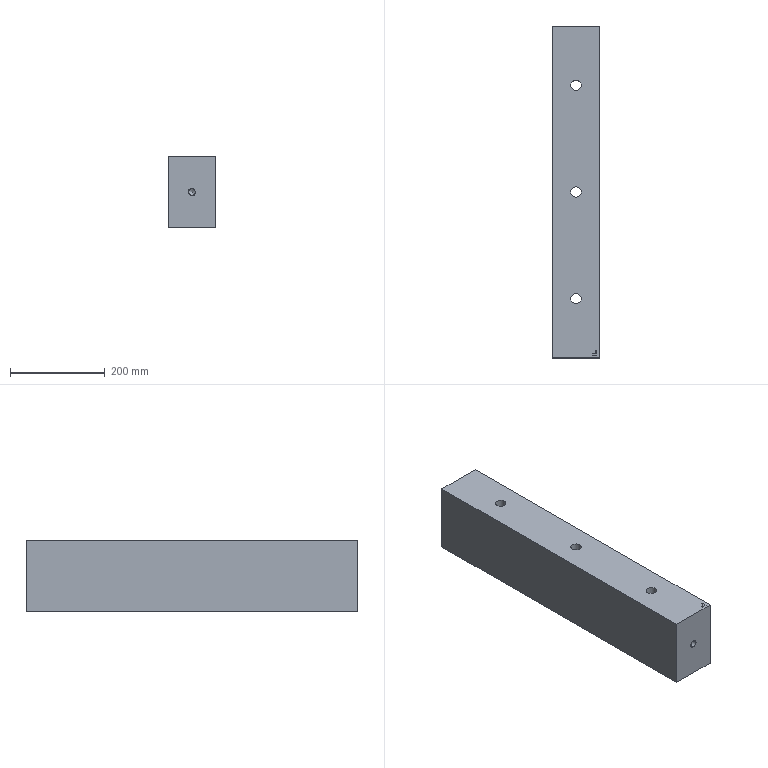Part | NX | features 模具.stp<1>[7] 2 | 1 solid | 48 faces | box 100 x 700 x 150 mm | volume 10309378 mm3 | plane 29 | cylinder 15 | cone 4 | commonest cylinder face diameters 22 x3 12.1 x2 13.7 x2 14 x2 14.1 x2 15.7 x2
STEP:
#1=CARTESIAN_POINT('',(-239.,-225.,-100.5));
#2=VERTEX_POINT('',#1);
#3=CARTESIAN_POINT('',(-250.,-225.,-100.5));
#4=DIRECTION('',(0.,0.,-1.));
#5=DIRECTION('',(1.,0.,0.));
#6=AXIS2_PLACEMENT_3D('',#3,#4,#5);
#7=CIRCLE('',#6,11.);
#8=EDGE_CURVE('',#2,#2,#7,.T.);
#9=ORIENTED_EDGE('',*,*,#8,.F.);
#10=EDGE_LOOP('',(#9));
#11=FACE_BOUND('',#10,.T.);
#12=CARTESIAN_POINT('',(-261.,-225.,-250.5));
#13=VERTEX_POINT('',#12);
#14=CARTESIAN_POINT('',(-250.,-225.,-250.5));
#15=DIRECTION('',(0.,0.,-1.));
#16=DIRECTION('',(-1.,0.,0.));
#17=AXIS2_PLACEMENT_3D('',#14,#15,#16);
#18=CIRCLE('',#17,11.);
#19=EDGE_CURVE('',#13,#13,#18,.T.);
#20=ORIENTED_EDGE('',*,*,#19,.T.);
#21=EDGE_LOOP('',(#20));
#22=FACE_BOUND('',#21,.T.);
#23=CARTESIAN_POINT('',(-250.,-225.,-100.5));
#24=DIRECTION('',(0.,0.,-1.));
#25=DIRECTION('',(1.,0.,0.));
#26=AXIS2_PLACEMENT_3D('',#23,#24,#25);
#27=CYLINDRICAL_SURFACE('',#26,11.);
#28=ADVANCED_FACE('',(#11,#22),#27,.F.);
#29=CARTESIAN_POINT('',(-239.,0.,-100.5));
#30=VERTEX_POINT('',#29);
#31=CARTESIAN_POINT('',(-250.,0.,-100.5));
#32=DIRECTION('',(0.,0.,-1.));
#33=DIRECTION('',(1.,0.,0.));
#34=AXIS2_PLACEMENT_3D('',#31,#32,#33);
#35=CIRCLE('',#34,11.);
#36=EDGE_CURVE('',#30,#30,#35,.T.);
#37=ORIENTED_EDGE('',*,*,#36,.F.);
#38=EDGE_LOOP('',(#37));
#39=FACE_BOUND('',#38,.T.);
#40=CARTESIAN_POINT('',(-261.,0.,-250.5));
#41=VERTEX_POINT('',#40);
#42=CARTESIAN_POINT('',(-250.,0.,-250.5));
#43=DIRECTION('',(0.,0.,-1.));
#44=DIRECTION('',(-1.,0.,0.));
#45=AXIS2_PLACEMENT_3D('',#42,#43,#44);
#46=CIRCLE('',#45,11.);
#47=EDGE_CURVE('',#41,#41,#46,.T.);
#48=ORIENTED_EDGE('',*,*,#47,.T.);
#49=EDGE_LOOP('',(#48));
#50=FACE_BOUND('',#49,.T.);
#51=CARTESIAN_POINT('',(-250.,0.,-100.5));
#52=DIRECTION('',(0.,0.,-1.));
#53=DIRECTION('',(1.,0.,0.));
#54=AXIS2_PLACEMENT_3D('',#51,#52,#53);
#55=CYLINDRICAL_SURFACE('',#54,11.);
#56=ADVANCED_FACE('',(#39,#50),#55,.F.);
#57=CARTESIAN_POINT('',(-239.,225.,-100.5));
#58=VERTEX_POINT('',#57);
#59=CARTESIAN_POINT('',(-250.,225.,-100.5));
#60=DIRECTION('',(0.,0.,-1.));
#61=DIRECTION('',(1.,0.,0.));
#62=AXIS2_PLACEMENT_3D('',#59,#60,#61);
#63=CIRCLE('',#62,11.);
#64=EDGE_CURVE('',#58,#58,#63,.T.);
#65=ORIENTED_EDGE('',*,*,#64,.F.);
#66=EDGE_LOOP('',(#65));
#67=FACE_BOUND('',#66,.T.);
#68=CARTESIAN_POINT('',(-261.,225.,-250.5));
#69=VERTEX_POINT('',#68);
#70=CARTESIAN_POINT('',(-250.,225.,-250.5));
#71=DIRECTION('',(0.,0.,-1.));
#72=DIRECTION('',(-1.,0.,0.));
#73=AXIS2_PLACEMENT_3D('',#70,#71,#72);
#74=CIRCLE('',#73,11.);
#75=EDGE_CURVE('',#69,#69,#74,.T.);
#76=ORIENTED_EDGE('',*,*,#75,.T.);
#77=EDGE_LOOP('',(#76));
#78=FACE_BOUND('',#77,.T.);
#79=CARTESIAN_POINT('',(-250.,225.,-100.5));
#80=DIRECTION('',(0.,0.,-1.));
#81=DIRECTION('',(1.,0.,0.));
#82=AXIS2_PLACEMENT_3D('',#79,#80,#81);
#83=CYLINDRICAL_SURFACE('',#82,11.);
#84=ADVANCED_FACE('',(#67,#78),#83,.F.);
#85=CARTESIAN_POINT('',(-250.,-297.,-215.505));
#86=VERTEX_POINT('',#85);
#87=VERTEX_LOOP('',#86);
#88=FACE_BOUND('',#87,.T.);
#89=CARTESIAN_POINT('',(-243.95,-297.,-218.998));
#90=VERTEX_POINT('',#89);
#91=CARTESIAN_POINT('',(-250.,-297.,-218.998));
#92=DIRECTION('',(0.,0.,1.));
#93=DIRECTION('',(1.,0.,0.));
#94=AXIS2_PLACEMENT_3D('',#91,#92,#93);
#95=CIRCLE('',#94,6.05);
#96=EDGE_CURVE('',#90,#90,#95,.T.);
#97=ORIENTED_EDGE('',*,*,#96,.F.);
#98=EDGE_LOOP('',(#97));
#99=FACE_BOUND('',#98,.T.);
#100=CARTESIAN_POINT('',(-250.,-297.,-216.505));
#101=DIRECTION('',(0.,0.,-1.));
#102=DIRECTION('',(1.,0.,0.));
#103=AXIS2_PLACEMENT_3D('',#100,#101,#102);
#104=CONICAL_SURFACE('',#103,1.732,1.047);
#105=ADVANCED_FACE('',(#88,#99),#104,.F.);
#106=CARTESIAN_POINT('',(-243.95,-297.,-222.5));
#107=VERTEX_POINT('',#106);
#108=CARTESIAN_POINT('',(-243.95,-297.,-223.5));
#109=VERTEX_POINT('',#108);
#110=CARTESIAN_POINT('',(-243.95,-297.,-218.998));
#111=DIRECTION('',(0.,0.,-1.));
#112=VECTOR('',#111,1000.);
#113=LINE('',#110,#112);
#114=EDGE_CURVE('',#107,#109,#113,.T.);
#115=ORIENTED_EDGE('',*,*,#114,.T.);
#116=CARTESIAN_POINT('',(-250.,-303.05,-223.5));
#117=VERTEX_POINT('',#116);
#118=CARTESIAN_POINT('',(-250.,-297.,-223.5));
#119=DIRECTION('',(0.,0.,1.));
#120=DIRECTION('',(0.,-1.,0.));
#121=AXIS2_PLACEMENT_3D('',#118,#119,#120);
#122=CIRCLE('',#121,6.05);
#123=EDGE_CURVE('',#109,#117,#122,.T.);
#124=ORIENTED_EDGE('',*,*,#123,.T.);
#125=CARTESIAN_POINT('',(-250.,-303.05,-222.5));
#126=VERTEX_POINT('',#125);
#127=CARTESIAN_POINT('',(-250.,-303.05,-218.998));
#128=DIRECTION('',(0.,0.,1.));
#129=VECTOR('',#128,1000.);
#130=LINE('',#127,#129);
#131=EDGE_CURVE('',#117,#126,#130,.T.);
#132=ORIENTED_EDGE('',*,*,#131,.T.);
#133=CARTESIAN_POINT('',(-250.,-297.,-222.5));
#134=DIRECTION('',(0.,0.,1.));
#135=DIRECTION('',(0.,-1.,0.));
#136=AXIS2_PLACEMENT_3D('',#133,#134,#135);
#137=CIRCLE('',#136,6.05);
#138=EDGE_CURVE('',#107,#126,#137,.T.);
#139=ORIENTED_EDGE('',*,*,#138,.F.);
#140=EDGE_LOOP('',(#115,#124,#132,#139));
#141=FACE_BOUND('',#140,.T.);
#142=ORIENTED_EDGE('',*,*,#96,.T.);
#143=EDGE_LOOP('',(#142));
#144=FACE_BOUND('',#143,.T.);
#145=CARTESIAN_POINT('',(-256.05,-297.,-250.5));
#146=VERTEX_POINT('',#145);
#147=CARTESIAN_POINT('',(-250.,-297.,-250.5));
#148=DIRECTION('',(0.,0.,-1.));
#149=DIRECTION('',(-1.,0.,0.));
#150=AXIS2_PLACEMENT_3D('',#147,#148,#149);
#151=CIRCLE('',#150,6.05);
#152=EDGE_CURVE('',#146,#146,#151,.T.);
#153=ORIENTED_EDGE('',*,*,#152,.T.);
#154=EDGE_LOOP('',(#153));
#155=FACE_BOUND('',#154,.T.);
#156=CARTESIAN_POINT('',(-250.,-297.,-218.998));
#157=DIRECTION('',(0.,0.,-1.));
#158=DIRECTION('',(1.,0.,0.));
#159=AXIS2_PLACEMENT_3D('',#156,#157,#158);
#160=CYLINDRICAL_SURFACE('',#159,6.05);
#161=ADVANCED_FACE('',(#141,#144,#155),#160,.F.);
#162=CARTESIAN_POINT('',(-250.,-304.,-222.5));
#163=VERTEX_POINT('',#162);
#164=CARTESIAN_POINT('',(-250.,-304.,-250.5));
#165=VERTEX_POINT('',#164);
#166=CARTESIAN_POINT('',(-250.,-304.,-222.5));
#167=DIRECTION('',(0.,0.,-1.));
#168=VECTOR('',#167,1000.);
#169=LINE('',#166,#168);
#170=EDGE_CURVE('',#163,#165,#169,.T.);
#171=ORIENTED_EDGE('',*,*,#170,.F.);
#172=CARTESIAN_POINT('',(-250.,-304.,-222.5));
#173=DIRECTION('',(0.,1.,0.));
#174=VECTOR('',#173,1000.);
#175=LINE('',#172,#174);
#176=EDGE_CURVE('',#163,#126,#175,.T.);
#177=ORIENTED_EDGE('',*,*,#176,.T.);
#178=ORIENTED_EDGE('',*,*,#131,.F.);
#179=CARTESIAN_POINT('',(-250.,-303.85,-223.5));
#180=VERTEX_POINT('',#179);
#181=CARTESIAN_POINT('',(-250.,-297.,-223.5));
#182=DIRECTION('',(0.,-1.,0.));
#183=VECTOR('',#182,1000.);
#184=LINE('',#181,#183);
#185=EDGE_CURVE('',#117,#180,#184,.T.);
#186=ORIENTED_EDGE('',*,*,#185,.T.);
#187=CARTESIAN_POINT('',(-250.,-303.85,-250.5));
#188=VERTEX_POINT('',#187);
#189=CARTESIAN_POINT('',(-250.,-303.85,-223.5));
#190=DIRECTION('',(0.,0.,-1.));
#191=VECTOR('',#190,1000.);
#192=LINE('',#189,#191);
#193=EDGE_CURVE('',#180,#188,#192,.T.);
#194=ORIENTED_EDGE('',*,*,#193,.T.);
#195=CARTESIAN_POINT('',(-250.,0.,-250.5));
#196=DIRECTION('',(0.,1.,0.));
#197=VECTOR('',#196,1000.);
#198=LINE('',#195,#197);
#199=EDGE_CURVE('',#165,#188,#198,.T.);
#200=ORIENTED_EDGE('',*,*,#199,.F.);
#201=EDGE_LOOP('',(#171,#177,#178,#186,#194,#200));
#202=FACE_BOUND('',#201,.T.);
#203=CARTESIAN_POINT('',(-250.,-304.,-222.5));
#204=DIRECTION('',(-1.,0.,0.));
#205=DIRECTION('',(0.,0.,1.));
#206=AXIS2_PLACEMENT_3D('',#203,#204,#205);
#207=PLANE('',#206);
#208=ADVANCED_FACE('',(#202),#207,.T.);
#209=CARTESIAN_POINT('',(-243.15,-297.,-250.5));
#210=VERTEX_POINT('',#209);
#211=CARTESIAN_POINT('',(-243.15,-297.,-223.5));
#212=VERTEX_POINT('',#211);
#213=CARTESIAN_POINT('',(-243.15,-297.,-223.5));
#214=DIRECTION('',(0.,0.,1.));
#215=VECTOR('',#214,1000.);
#216=LINE('',#213,#215);
#217=EDGE_CURVE('',#210,#212,#216,.T.);
#218=ORIENTED_EDGE('',*,*,#217,.T.);
#219=CARTESIAN_POINT('',(-250.,-297.,-223.5));
#220=DIRECTION('',(-1.,0.,0.));
#221=VECTOR('',#220,1000.);
#222=LINE('',#219,#221);
#223=EDGE_CURVE('',#212,#109,#222,.T.);
#224=ORIENTED_EDGE('',*,*,#223,.T.);
#225=ORIENTED_EDGE('',*,*,#114,.F.);
#226=CARTESIAN_POINT('',(-243.,-297.,-222.5));
#227=VERTEX_POINT('',#226);
#228=CARTESIAN_POINT('',(-243.,-297.,-222.5));
#229=DIRECTION('',(1.,0.,0.));
#230=VECTOR('',#229,1000.);
#231=LINE('',#228,#230);
#232=EDGE_CURVE('',#107,#227,#231,.T.);
#233=ORIENTED_EDGE('',*,*,#232,.T.);
#234=CARTESIAN_POINT('',(-243.,-297.,-250.5));
#235=VERTEX_POINT('',#234);
#236=CARTESIAN_POINT('',(-243.,-297.,-222.5));
#237=DIRECTION('',(0.,0.,1.));
#238=VECTOR('',#237,1000.);
#239=LINE('',#236,#238);
#240=EDGE_CURVE('',#235,#227,#239,.T.);
#241=ORIENTED_EDGE('',*,*,#240,.F.);
#242=CARTESIAN_POINT('',(-250.,-297.,-250.5));
#243=DIRECTION('',(1.,0.,0.));
#244=VECTOR('',#243,1000.);
#245=LINE('',#242,#244);
#246=EDGE_CURVE('',#210,#235,#245,.T.);
#247=ORIENTED_EDGE('',*,*,#246,.F.);
#248=EDGE_LOOP('',(#218,#224,#225,#233,#241,#247));
#249=FACE_BOUND('',#248,.T.);
#250=CARTESIAN_POINT('',(-243.,-297.,-222.5));
#251=DIRECTION('',(0.,1.,0.));
#252=DIRECTION('',(0.,0.,-1.));
#253=AXIS2_PLACEMENT_3D('',#250,#251,#252);
#254=PLANE('',#253);
#255=ADVANCED_FACE('',(#249),#254,.T.);
#256=ORIENTED_EDGE('',*,*,#193,.F.);
#257=CARTESIAN_POINT('',(-250.,-297.,-223.5));
#258=DIRECTION('',(0.,0.,-1.));
#259=DIRECTION('',(1.,0.,0.));
#260=AXIS2_PLACEMENT_3D('',#257,#258,#259);
#261=CIRCLE('',#260,6.85);
#262=EDGE_CURVE('',#180,#212,#261,.T.);
#263=ORIENTED_EDGE('',*,*,#262,.T.);
#264=ORIENTED_EDGE('',*,*,#217,.F.);
#265=CARTESIAN_POINT('',(-250.,-297.,-250.5));
#266=DIRECTION('',(0.,0.,-1.));
#267=DIRECTION('',(-1.,0.,0.));
#268=AXIS2_PLACEMENT_3D('',#265,#266,#267);
#269=CIRCLE('',#268,6.85);
#270=EDGE_CURVE('',#188,#210,#269,.T.);
#271=ORIENTED_EDGE('',*,*,#270,.F.);
#272=EDGE_LOOP('',(#256,#263,#264,#271));
#273=FACE_BOUND('',#272,.T.);
#274=CARTESIAN_POINT('',(-250.,-297.,-223.5));
#275=DIRECTION('',(0.,0.,-1.));
#276=DIRECTION('',(1.,0.,0.));
#277=AXIS2_PLACEMENT_3D('',#274,#275,#276);
#278=CYLINDRICAL_SURFACE('',#277,6.85);
#279=ADVANCED_FACE('',(#273),#278,.T.);
#280=ORIENTED_EDGE('',*,*,#223,.F.);
#281=ORIENTED_EDGE('',*,*,#262,.F.);
#282=ORIENTED_EDGE('',*,*,#185,.F.);
#283=ORIENTED_EDGE('',*,*,#123,.F.);
#284=EDGE_LOOP('',(#280,#281,#282,#283));
#285=FACE_BOUND('',#284,.T.);
#286=CARTESIAN_POINT('',(-250.,-297.,-223.5));
#287=DIRECTION('',(0.,0.,1.));
#288=DIRECTION('',(0.,-1.,0.));
#289=AXIS2_PLACEMENT_3D('',#286,#287,#288);
#290=PLANE('',#289);
#291=ADVANCED_FACE('',(#285),#290,.T.);
#292=CARTESIAN_POINT('',(-250.,-297.,-250.5));
#293=DIRECTION('',(0.,0.,-1.));
#294=DIRECTION('',(-1.,0.,0.));
#295=AXIS2_PLACEMENT_3D('',#292,#293,#294);
#296=CIRCLE('',#295,7.);
#297=EDGE_CURVE('',#165,#235,#296,.T.);
#298=ORIENTED_EDGE('',*,*,#297,.T.);
#299=ORIENTED_EDGE('',*,*,#240,.T.);
#300=CARTESIAN_POINT('',(-250.,-297.,-222.5));
#301=DIRECTION('',(0.,0.,-1.));
#302=DIRECTION('',(1.,0.,0.));
#303=AXIS2_PLACEMENT_3D('',#300,#301,#302);
#304=CIRCLE('',#303,7.);
#305=EDGE_CURVE('',#163,#227,#304,.T.);
#306=ORIENTED_EDGE('',*,*,#305,.F.);
#307=ORIENTED_EDGE('',*,*,#170,.T.);
#308=EDGE_LOOP('',(#298,#299,#306,#307));
#309=FACE_BOUND('',#308,.T.);
#310=CARTESIAN_POINT('',(-250.,-297.,-222.5));
#311=DIRECTION('',(0.,0.,-1.));
#312=DIRECTION('',(1.,0.,0.));
#313=AXIS2_PLACEMENT_3D('',#310,#311,#312);
#314=CYLINDRICAL_SURFACE('',#313,7.);
#315=ADVANCED_FACE('',(#309),#314,.F.);
#316=ORIENTED_EDGE('',*,*,#138,.T.);
#317=ORIENTED_EDGE('',*,*,#176,.F.);
#318=ORIENTED_EDGE('',*,*,#305,.T.);
#319=ORIENTED_EDGE('',*,*,#232,.F.);
#320=EDGE_LOOP('',(#316,#317,#318,#319));
#321=FACE_BOUND('',#320,.T.);
#322=CARTESIAN_POINT('',(-250.,-297.,-222.5));
#323=DIRECTION('',(0.,0.,1.));
#324=DIRECTION('',(0.,-1.,0.));
#325=AXIS2_PLACEMENT_3D('',#322,#323,#324);
#326=PLANE('',#325);
#327=ADVANCED_FACE('',(#321),#326,.F.);
#328=CARTESIAN_POINT('',(-250.,297.,-215.505));
#329=VERTEX_POINT('',#328);
#330=VERTEX_LOOP('',#329);
#331=FACE_BOUND('',#330,.T.);
#332=CARTESIAN_POINT('',(-243.95,297.,-218.998));
#333=VERTEX_POINT('',#332);
#334=CARTESIAN_POINT('',(-250.,297.,-218.998));
#335=DIRECTION('',(0.,0.,1.));
#336=DIRECTION('',(1.,0.,0.));
#337=AXIS2_PLACEMENT_3D('',#334,#335,#336);
#338=CIRCLE('',#337,6.05);
#339=EDGE_CURVE('',#333,#333,#338,.T.);
#340=ORIENTED_EDGE('',*,*,#339,.F.);
#341=EDGE_LOOP('',(#340));
#342=FACE_BOUND('',#341,.T.);
#343=CARTESIAN_POINT('',(-250.,297.,-216.505));
#344=DIRECTION('',(0.,0.,-1.));
#345=DIRECTION('',(1.,0.,0.));
#346=AXIS2_PLACEMENT_3D('',#343,#344,#345);
#347=CONICAL_SURFACE('',#346,1.732,1.047);
#348=ADVANCED_FACE('',(#331,#342),#347,.F.);
#349=CARTESIAN_POINT('',(-243.95,297.,-222.5));
#350=VERTEX_POINT('',#349);
#351=CARTESIAN_POINT('',(-243.95,297.,-223.5));
#352=VERTEX_POINT('',#351);
#353=CARTESIAN_POINT('',(-243.95,297.,-218.998));
#354=DIRECTION('',(0.,0.,-1.));
#355=VECTOR('',#354,1000.);
#356=LINE('',#353,#355);
#357=EDGE_CURVE('',#350,#352,#356,.T.);
#358=ORIENTED_EDGE('',*,*,#357,.T.);
#359=CARTESIAN_POINT('',(-250.,290.95,-223.5));
#360=VERTEX_POINT('',#359);
#361=CARTESIAN_POINT('',(-250.,297.,-223.5));
#362=DIRECTION('',(0.,0.,1.));
#363=DIRECTION('',(0.,-1.,0.));
#364=AXIS2_PLACEMENT_3D('',#361,#362,#363);
#365=CIRCLE('',#364,6.05);
#366=EDGE_CURVE('',#352,#360,#365,.T.);
#367=ORIENTED_EDGE('',*,*,#366,.T.);
#368=CARTESIAN_POINT('',(-250.,290.95,-222.5));
#369=VERTEX_POINT('',#368);
#370=CARTESIAN_POINT('',(-250.,290.95,-218.998));
#371=DIRECTION('',(0.,0.,1.));
#372=VECTOR('',#371,1000.);
#373=LINE('',#370,#372);
#374=EDGE_CURVE('',#360,#369,#373,.T.);
#375=ORIENTED_EDGE('',*,*,#374,.T.);
#376=CARTESIAN_POINT('',(-250.,297.,-222.5));
#377=DIRECTION('',(0.,0.,1.));
#378=DIRECTION('',(0.,-1.,0.));
#379=AXIS2_PLACEMENT_3D('',#376,#377,#378);
#380=CIRCLE('',#379,6.05);
#381=EDGE_CURVE('',#350,#369,#380,.T.);
#382=ORIENTED_EDGE('',*,*,#381,.F.);
#383=EDGE_LOOP('',(#358,#367,#375,#382));
#384=FACE_BOUND('',#383,.T.);
#385=ORIENTED_EDGE('',*,*,#339,.T.);
#386=EDGE_LOOP('',(#385));
#387=FACE_BOUND('',#386,.T.);
#388=CARTESIAN_POINT('',(-256.05,297.,-250.5));
#389=VERTEX_POINT('',#388);
#390=CARTESIAN_POINT('',(-250.,297.,-250.5));
#391=DIRECTION('',(0.,0.,-1.));
#392=DIRECTION('',(-1.,0.,0.));
#393=AXIS2_PLACEMENT_3D('',#390,#391,#392);
#394=CIRCLE('',#393,6.05);
#395=EDGE_CURVE('',#389,#389,#394,.T.);
#396=ORIENTED_EDGE('',*,*,#395,.T.);
#397=EDGE_LOOP('',(#396));
#398=FACE_BOUND('',#397,.T.);
#399=CARTESIAN_POINT('',(-250.,297.,-218.998));
#400=DIRECTION('',(0.,0.,-1.));
#401=DIRECTION('',(1.,0.,0.));
#402=AXIS2_PLACEMENT_3D('',#399,#400,#401);
#403=CYLINDRICAL_SURFACE('',#402,6.05);
#404=ADVANCED_FACE('',(#384,#387,#398),#403,.F.);
#405=CARTESIAN_POINT('',(-250.,290.,-222.5));
#406=VERTEX_POINT('',#405);
#407=CARTESIAN_POINT('',(-250.,290.,-250.5));
#408=VERTEX_POINT('',#407);
#409=CARTESIAN_POINT('',(-250.,290.,-222.5));
#410=DIRECTION('',(0.,0.,-1.));
#411=VECTOR('',#410,1000.);
#412=LINE('',#409,#411);
#413=EDGE_CURVE('',#406,#408,#412,.T.);
#414=ORIENTED_EDGE('',*,*,#413,.F.);
#415=CARTESIAN_POINT('',(-250.,290.,-222.5));
#416=DIRECTION('',(0.,1.,0.));
#417=VECTOR('',#416,1000.);
#418=LINE('',#415,#417);
#419=EDGE_CURVE('',#406,#369,#418,.T.);
#420=ORIENTED_EDGE('',*,*,#419,.T.);
#421=ORIENTED_EDGE('',*,*,#374,.F.);
#422=CARTESIAN_POINT('',(-250.,290.15,-223.5));
#423=VERTEX_POINT('',#422);
#424=CARTESIAN_POINT('',(-250.,297.,-223.5));
#425=DIRECTION('',(0.,-1.,0.));
#426=VECTOR('',#425,1000.);
#427=LINE('',#424,#426);
#428=EDGE_CURVE('',#360,#423,#427,.T.);
#429=ORIENTED_EDGE('',*,*,#428,.T.);
#430=CARTESIAN_POINT('',(-250.,290.15,-250.5));
#431=VERTEX_POINT('',#430);
#432=CARTESIAN_POINT('',(-250.,290.15,-223.5));
#433=DIRECTION('',(0.,0.,-1.));
#434=VECTOR('',#433,1000.);
#435=LINE('',#432,#434);
#436=EDGE_CURVE('',#423,#431,#435,.T.);
#437=ORIENTED_EDGE('',*,*,#436,.T.);
#438=CARTESIAN_POINT('',(-250.,0.,-250.5));
#439=DIRECTION('',(0.,1.,0.));
#440=VECTOR('',#439,1000.);
#441=LINE('',#438,#440);
#442=EDGE_CURVE('',#408,#431,#441,.T.);
#443=ORIENTED_EDGE('',*,*,#442,.F.);
#444=EDGE_LOOP('',(#414,#420,#421,#429,#437,#443));
#445=FACE_BOUND('',#444,.T.);
#446=CARTESIAN_POINT('',(-250.,290.,-222.5));
#447=DIRECTION('',(-1.,0.,0.));
#448=DIRECTION('',(0.,0.,1.));
#449=AXIS2_PLACEMENT_3D('',#446,#447,#448);
#450=PLANE('',#449);
#451=ADVANCED_FACE('',(#445),#450,.T.);
#452=CARTESIAN_POINT('',(-243.15,297.,-250.5));
#453=VERTEX_POINT('',#452);
#454=CARTESIAN_POINT('',(-243.15,297.,-223.5));
#455=VERTEX_POINT('',#454);
#456=CARTESIAN_POINT('',(-243.15,297.,-223.5));
#457=DIRECTION('',(0.,0.,1.));
#458=VECTOR('',#457,1000.);
#459=LINE('',#456,#458);
#460=EDGE_CURVE('',#453,#455,#459,.T.);
#461=ORIENTED_EDGE('',*,*,#460,.T.);
#462=CARTESIAN_POINT('',(-250.,297.,-223.5));
#463=DIRECTION('',(-1.,0.,0.));
#464=VECTOR('',#463,1000.);
#465=LINE('',#462,#464);
#466=EDGE_CURVE('',#455,#352,#465,.T.);
#467=ORIENTED_EDGE('',*,*,#466,.T.);
#468=ORIENTED_EDGE('',*,*,#357,.F.);
#469=CARTESIAN_POINT('',(-243.,297.,-222.5));
#470=VERTEX_POINT('',#469);
#471=CARTESIAN_POINT('',(-243.,297.,-222.5));
#472=DIRECTION('',(1.,0.,0.));
#473=VECTOR('',#472,1000.);
#474=LINE('',#471,#473);
#475=EDGE_CURVE('',#350,#470,#474,.T.);
#476=ORIENTED_EDGE('',*,*,#475,.T.);
#477=CARTESIAN_POINT('',(-243.,297.,-250.5));
#478=VERTEX_POINT('',#477);
#479=CARTESIAN_POINT('',(-243.,297.,-222.5));
#480=DIRECTION('',(0.,0.,1.));
#481=VECTOR('',#480,1000.);
#482=LINE('',#479,#481);
#483=EDGE_CURVE('',#478,#470,#482,.T.);
#484=ORIENTED_EDGE('',*,*,#483,.F.);
#485=CARTESIAN_POINT('',(-250.,297.,-250.5));
#486=DIRECTION('',(1.,0.,0.));
#487=VECTOR('',#486,1000.);
#488=LINE('',#485,#487);
#489=EDGE_CURVE('',#453,#478,#488,.T.);
#490=ORIENTED_EDGE('',*,*,#489,.F.);
#491=EDGE_LOOP('',(#461,#467,#468,#476,#484,#490));
#492=FACE_BOUND('',#491,.T.);
#493=CARTESIAN_POINT('',(-243.,297.,-222.5));
#494=DIRECTION('',(0.,1.,0.));
#495=DIRECTION('',(0.,0.,-1.));
#496=AXIS2_PLACEMENT_3D('',#493,#494,#495);
#497=PLANE('',#496);
#498=ADVANCED_FACE('',(#492),#497,.T.);
#499=ORIENTED_EDGE('',*,*,#436,.F.);
#500=CARTESIAN_POINT('',(-250.,297.,-223.5));
#501=DIRECTION('',(0.,0.,-1.));
#502=DIRECTION('',(1.,0.,0.));
#503=AXIS2_PLACEMENT_3D('',#500,#501,#502);
#504=CIRCLE('',#503,6.85);
#505=EDGE_CURVE('',#423,#455,#504,.T.);
#506=ORIENTED_EDGE('',*,*,#505,.T.);
#507=ORIENTED_EDGE('',*,*,#460,.F.);
#508=CARTESIAN_POINT('',(-250.,297.,-250.5));
#509=DIRECTION('',(0.,0.,-1.));
#510=DIRECTION('',(-1.,0.,0.));
#511=AXIS2_PLACEMENT_3D('',#508,#509,#510);
#512=CIRCLE('',#511,6.85);
#513=EDGE_CURVE('',#431,#453,#512,.T.);
#514=ORIENTED_EDGE('',*,*,#513,.F.);
#515=EDGE_LOOP('',(#499,#506,#507,#514));
#516=FACE_BOUND('',#515,.T.);
#517=CARTESIAN_POINT('',(-250.,297.,-223.5));
#518=DIRECTION('',(0.,0.,-1.));
#519=DIRECTION('',(1.,0.,0.));
#520=AXIS2_PLACEMENT_3D('',#517,#518,#519);
#521=CYLINDRICAL_SURFACE('',#520,6.85);
#522=ADVANCED_FACE('',(#516),#521,.T.);
#523=ORIENTED_EDGE('',*,*,#466,.F.);
#524=ORIENTED_EDGE('',*,*,#505,.F.);
#525=ORIENTED_EDGE('',*,*,#428,.F.);
#526=ORIENTED_EDGE('',*,*,#366,.F.);
#527=EDGE_LOOP('',(#523,#524,#525,#526));
#528=FACE_BOUND('',#527,.T.);
#529=CARTESIAN_POINT('',(-250.,297.,-223.5));
#530=DIRECTION('',(0.,0.,1.));
#531=DIRECTION('',(0.,-1.,0.));
#532=AXIS2_PLACEMENT_3D('',#529,#530,#531);
#533=PLANE('',#532);
#534=ADVANCED_FACE('',(#528),#533,.T.);
#535=CARTESIAN_POINT('',(-250.,297.,-250.5));
#536=DIRECTION('',(0.,0.,-1.));
#537=DIRECTION('',(-1.,0.,0.));
#538=AXIS2_PLACEMENT_3D('',#535,#536,#537);
#539=CIRCLE('',#538,7.);
#540=EDGE_CURVE('',#408,#478,#539,.T.);
#541=ORIENTED_EDGE('',*,*,#540,.T.);
#542=ORIENTED_EDGE('',*,*,#483,.T.);
#543=CARTESIAN_POINT('',(-250.,297.,-222.5));
#544=DIRECTION('',(0.,0.,-1.));
#545=DIRECTION('',(1.,0.,0.));
#546=AXIS2_PLACEMENT_3D('',#543,#544,#545);
#547=CIRCLE('',#546,7.);
#548=EDGE_CURVE('',#406,#470,#547,.T.);
#549=ORIENTED_EDGE('',*,*,#548,.F.);
#550=ORIENTED_EDGE('',*,*,#413,.T.);
#551=EDGE_LOOP('',(#541,#542,#549,#550));
#552=FACE_BOUND('',#551,.T.);
#553=CARTESIAN_POINT('',(-250.,297.,-222.5));
#554=DIRECTION('',(0.,0.,-1.));
#555=DIRECTION('',(1.,0.,0.));
#556=AXIS2_PLACEMENT_3D('',#553,#554,#555);
#557=CYLINDRICAL_SURFACE('',#556,7.);
#558=ADVANCED_FACE('',(#552),#557,.F.);
#559=ORIENTED_EDGE('',*,*,#381,.T.);
#560=ORIENTED_EDGE('',*,*,#419,.F.);
#561=ORIENTED_EDGE('',*,*,#548,.T.);
#562=ORIENTED_EDGE('',*,*,#475,.F.);
#563=EDGE_LOOP('',(#559,#560,#561,#562));
#564=FACE_BOUND('',#563,.T.);
#565=CARTESIAN_POINT('',(-250.,297.,-222.5));
#566=DIRECTION('',(0.,0.,1.));
#567=DIRECTION('',(0.,-1.,0.));
#568=AXIS2_PLACEMENT_3D('',#565,#566,#567);
#569=PLANE('',#568);
#570=ADVANCED_FACE('',(#564),#569,.F.);
#571=CARTESIAN_POINT('',(-250.,-311.005,-175.5));
#572=VERTEX_POINT('',#571);
#573=VERTEX_LOOP('',#572);
#574=FACE_BOUND('',#573,.T.);
#575=CARTESIAN_POINT('',(-242.95,-315.075,-175.5));
#576=VERTEX_POINT('',#575);
#577=CARTESIAN_POINT('',(-250.,-315.075,-175.5));
#578=DIRECTION('',(0.,1.,0.));
#579=DIRECTION('',(1.,0.,0.));
#580=AXIS2_PLACEMENT_3D('',#577,#578,#579);
#581=CIRCLE('',#580,7.05);
#582=EDGE_CURVE('',#576,#576,#581,.T.);
#583=ORIENTED_EDGE('',*,*,#582,.F.);
#584=EDGE_LOOP('',(#583));
#585=FACE_BOUND('',#584,.T.);
#586=CARTESIAN_POINT('',(-250.,-312.005,-175.5));
#587=DIRECTION('',(0.,-1.,0.));
#588=DIRECTION('',(1.,0.,0.));
#589=AXIS2_PLACEMENT_3D('',#586,#587,#588);
#590=CONICAL_SURFACE('',#589,1.732,1.047);
#591=ADVANCED_FACE('',(#574,#585),#590,.F.);
#592=CARTESIAN_POINT('',(-242.95,-321.,-175.5));
#593=VERTEX_POINT('',#592);
#594=CARTESIAN_POINT('',(-242.95,-322.,-175.5));
#595=VERTEX_POINT('',#594);
#596=CARTESIAN_POINT('',(-242.95,-315.075,-175.5));
#597=DIRECTION('',(0.,-1.,0.));
#598=VECTOR('',#597,1000.);
#599=LINE('',#596,#598);
#600=EDGE_CURVE('',#593,#595,#599,.T.);
#601=ORIENTED_EDGE('',*,*,#600,.T.);
#602=CARTESIAN_POINT('',(-250.,-322.,-168.45));
#603=VERTEX_POINT('',#602);
#604=CARTESIAN_POINT('',(-250.,-322.,-175.5));
#605=DIRECTION('',(0.,1.,0.));
#606=DIRECTION('',(0.,0.,1.));
#607=AXIS2_PLACEMENT_3D('',#604,#605,#606);
#608=CIRCLE('',#607,7.05);
#609=EDGE_CURVE('',#595,#603,#608,.T.);
#610=ORIENTED_EDGE('',*,*,#609,.T.);
#611=CARTESIAN_POINT('',(-250.,-321.,-168.45));
#612=VERTEX_POINT('',#611);
#613=CARTESIAN_POINT('',(-250.,-315.075,-168.45));
#614=DIRECTION('',(0.,1.,0.));
#615=VECTOR('',#614,1000.);
#616=LINE('',#613,#615);
#617=EDGE_CURVE('',#603,#612,#616,.T.);
#618=ORIENTED_EDGE('',*,*,#617,.T.);
#619=CARTESIAN_POINT('',(-250.,-321.,-175.5));
#620=DIRECTION('',(0.,1.,0.));
#621=DIRECTION('',(0.,0.,1.));
#622=AXIS2_PLACEMENT_3D('',#619,#620,#621);
#623=CIRCLE('',#622,7.05);
#624=EDGE_CURVE('',#593,#612,#623,.T.);
#625=ORIENTED_EDGE('',*,*,#624,.F.);
#626=EDGE_LOOP('',(#601,#610,#618,#625));
#627=FACE_BOUND('',#626,.T.);
#628=ORIENTED_EDGE('',*,*,#582,.T.);
#629=EDGE_LOOP('',(#628));
#630=FACE_BOUND('',#629,.T.);
#631=CARTESIAN_POINT('',(-250.,-350.,-182.55));
#632=VERTEX_POINT('',#631);
#633=CARTESIAN_POINT('',(-250.,-350.,-175.5));
#634=DIRECTION('',(0.,-1.,0.));
#635=DIRECTION('',(0.,0.,-1.));
#636=AXIS2_PLACEMENT_3D('',#633,#634,#635);
#637=CIRCLE('',#636,7.05);
#638=EDGE_CURVE('',#632,#632,#637,.T.);
#639=ORIENTED_EDGE('',*,*,#638,.T.);
#640=EDGE_LOOP('',(#639));
#641=FACE_BOUND('',#640,.T.);
#642=CARTESIAN_POINT('',(-250.,-315.075,-175.5));
#643=DIRECTION('',(0.,-1.,0.));
#644=DIRECTION('',(1.,0.,0.));
#645=AXIS2_PLACEMENT_3D('',#642,#643,#644);
#646=CYLINDRICAL_SURFACE('',#645,7.05);
#647=ADVANCED_FACE('',(#627,#630,#641),#646,.F.);
#648=CARTESIAN_POINT('',(-250.,-321.,-167.5));
#649=VERTEX_POINT('',#648);
#650=CARTESIAN_POINT('',(-250.,-350.,-167.5));
#651=VERTEX_POINT('',#650);
#652=CARTESIAN_POINT('',(-250.,-321.,-167.5));
#653=DIRECTION('',(0.,-1.,0.));
#654=VECTOR('',#653,1000.);
#655=LINE('',#652,#654);
#656=EDGE_CURVE('',#649,#651,#655,.T.);
#657=ORIENTED_EDGE('',*,*,#656,.F.);
#658=CARTESIAN_POINT('',(-250.,-321.,-167.5));
#659=DIRECTION('',(0.,0.,-1.));
#660=VECTOR('',#659,1000.);
#661=LINE('',#658,#660);
#662=EDGE_CURVE('',#649,#612,#661,.T.);
#663=ORIENTED_EDGE('',*,*,#662,.T.);
#664=ORIENTED_EDGE('',*,*,#617,.F.);
#665=CARTESIAN_POINT('',(-250.,-322.,-167.65));
#666=VERTEX_POINT('',#665);
#667=CARTESIAN_POINT('',(-250.,-322.,-175.5));
#668=DIRECTION('',(0.,0.,1.));
#669=VECTOR('',#668,1000.);
#670=LINE('',#667,#669);
#671=EDGE_CURVE('',#603,#666,#670,.T.);
#672=ORIENTED_EDGE('',*,*,#671,.T.);
#673=CARTESIAN_POINT('',(-250.,-350.,-167.65));
#674=VERTEX_POINT('',#673);
#675=CARTESIAN_POINT('',(-250.,-322.,-167.65));
#676=DIRECTION('',(0.,-1.,0.));
#677=VECTOR('',#676,1000.);
#678=LINE('',#675,#677);
#679=EDGE_CURVE('',#666,#674,#678,.T.);
#680=ORIENTED_EDGE('',*,*,#679,.T.);
#681=CARTESIAN_POINT('',(-250.,-350.,-250.5));
#682=DIRECTION('',(0.,0.,-1.));
#683=VECTOR('',#682,1000.);
#684=LINE('',#681,#683);
#685=EDGE_CURVE('',#651,#674,#684,.T.);
#686=ORIENTED_EDGE('',*,*,#685,.F.);
#687=EDGE_LOOP('',(#657,#663,#664,#672,#680,#686));
#688=FACE_BOUND('',#687,.T.);
#689=CARTESIAN_POINT('',(-250.,-321.,-167.5));
#690=DIRECTION('',(-1.,0.,0.));
#691=DIRECTION('',(0.,0.,1.));
#692=AXIS2_PLACEMENT_3D('',#689,#690,#691);
#693=PLANE('',#692);
#694=ADVANCED_FACE('',(#688),#693,.T.);
#695=CARTESIAN_POINT('',(-242.15,-350.,-175.5));
#696=VERTEX_POINT('',#695);
#697=CARTESIAN_POINT('',(-242.15,-322.,-175.5));
#698=VERTEX_POINT('',#697);
#699=CARTESIAN_POINT('',(-242.15,-322.,-175.5));
#700=DIRECTION('',(0.,1.,0.));
#701=VECTOR('',#700,1000.);
#702=LINE('',#699,#701);
#703=EDGE_CURVE('',#696,#698,#702,.T.);
#704=ORIENTED_EDGE('',*,*,#703,.T.);
#705=CARTESIAN_POINT('',(-250.,-322.,-175.5));
#706=DIRECTION('',(-1.,0.,0.));
#707=VECTOR('',#706,1000.);
#708=LINE('',#705,#707);
#709=EDGE_CURVE('',#698,#595,#708,.T.);
#710=ORIENTED_EDGE('',*,*,#709,.T.);
#711=ORIENTED_EDGE('',*,*,#600,.F.);
#712=CARTESIAN_POINT('',(-242.,-321.,-175.5));
#713=VERTEX_POINT('',#712);
#714=CARTESIAN_POINT('',(-242.,-321.,-175.5));
#715=DIRECTION('',(1.,0.,0.));
#716=VECTOR('',#715,1000.);
#717=LINE('',#714,#716);
#718=EDGE_CURVE('',#593,#713,#717,.T.);
#719=ORIENTED_EDGE('',*,*,#718,.T.);
#720=CARTESIAN_POINT('',(-242.,-350.,-175.5));
#721=VERTEX_POINT('',#720);
#722=CARTESIAN_POINT('',(-242.,-321.,-175.5));
#723=DIRECTION('',(0.,1.,0.));
#724=VECTOR('',#723,1000.);
#725=LINE('',#722,#724);
#726=EDGE_CURVE('',#721,#713,#725,.T.);
#727=ORIENTED_EDGE('',*,*,#726,.F.);
#728=CARTESIAN_POINT('',(-250.,-350.,-175.5));
#729=DIRECTION('',(1.,0.,0.));
#730=VECTOR('',#729,1000.);
#731=LINE('',#728,#730);
#732=EDGE_CURVE('',#696,#721,#731,.T.);
#733=ORIENTED_EDGE('',*,*,#732,.F.);
#734=EDGE_LOOP('',(#704,#710,#711,#719,#727,#733));
#735=FACE_BOUND('',#734,.T.);
#736=CARTESIAN_POINT('',(-242.,-321.,-175.5));
#737=DIRECTION('',(0.,0.,-1.));
#738=DIRECTION('',(0.,-1.,0.));
#739=AXIS2_PLACEMENT_3D('',#736,#737,#738);
#740=PLANE('',#739);
#741=ADVANCED_FACE('',(#735),#740,.T.);
#742=ORIENTED_EDGE('',*,*,#679,.F.);
#743=CARTESIAN_POINT('',(-250.,-322.,-175.5));
#744=DIRECTION('',(0.,-1.,0.));
#745=DIRECTION('',(1.,0.,0.));
#746=AXIS2_PLACEMENT_3D('',#743,#744,#745);
#747=CIRCLE('',#746,7.85);
#748=EDGE_CURVE('',#666,#698,#747,.T.);
#749=ORIENTED_EDGE('',*,*,#748,.T.);
#750=ORIENTED_EDGE('',*,*,#703,.F.);
#751=CARTESIAN_POINT('',(-250.,-350.,-175.5));
#752=DIRECTION('',(0.,-1.,0.));
#753=DIRECTION('',(0.,0.,-1.));
#754=AXIS2_PLACEMENT_3D('',#751,#752,#753);
#755=CIRCLE('',#754,7.85);
#756=EDGE_CURVE('',#674,#696,#755,.T.);
#757=ORIENTED_EDGE('',*,*,#756,.F.);
#758=EDGE_LOOP('',(#742,#749,#750,#757));
#759=FACE_BOUND('',#758,.T.);
#760=CARTESIAN_POINT('',(-250.,-322.,-175.5));
#761=DIRECTION('',(0.,-1.,0.));
#762=DIRECTION('',(1.,0.,0.));
#763=AXIS2_PLACEMENT_3D('',#760,#761,#762);
#764=CYLINDRICAL_SURFACE('',#763,7.85);
#765=ADVANCED_FACE('',(#759),#764,.T.);
#766=ORIENTED_EDGE('',*,*,#709,.F.);
#767=ORIENTED_EDGE('',*,*,#748,.F.);
#768=ORIENTED_EDGE('',*,*,#671,.F.);
#769=ORIENTED_EDGE('',*,*,#609,.F.);
#770=EDGE_LOOP('',(#766,#767,#768,#769));
#771=FACE_BOUND('',#770,.T.);
#772=CARTESIAN_POINT('',(-250.,-322.,-175.5));
#773=DIRECTION('',(0.,1.,0.));
#774=DIRECTION('',(0.,0.,-1.));
#775=AXIS2_PLACEMENT_3D('',#772,#773,#774);
#776=PLANE('',#775);
#777=ADVANCED_FACE('',(#771),#776,.T.);
#778=CARTESIAN_POINT('',(-250.,-350.,-175.5));
#779=DIRECTION('',(0.,-1.,0.));
#780=DIRECTION('',(0.,0.,-1.));
#781=AXIS2_PLACEMENT_3D('',#778,#779,#780);
#782=CIRCLE('',#781,8.);
#783=EDGE_CURVE('',#651,#721,#782,.T.);
#784=ORIENTED_EDGE('',*,*,#783,.T.);
#785=ORIENTED_EDGE('',*,*,#726,.T.);
#786=CARTESIAN_POINT('',(-250.,-321.,-175.5));
#787=DIRECTION('',(0.,-1.,0.));
#788=DIRECTION('',(1.,0.,0.));
#789=AXIS2_PLACEMENT_3D('',#786,#787,#788);
#790=CIRCLE('',#789,8.);
#791=EDGE_CURVE('',#649,#713,#790,.T.);
#792=ORIENTED_EDGE('',*,*,#791,.F.);
#793=ORIENTED_EDGE('',*,*,#656,.T.);
#794=EDGE_LOOP('',(#784,#785,#792,#793));
#795=FACE_BOUND('',#794,.T.);
#796=CARTESIAN_POINT('',(-250.,-321.,-175.5));
#797=DIRECTION('',(0.,-1.,0.));
#798=DIRECTION('',(1.,0.,0.));
#799=AXIS2_PLACEMENT_3D('',#796,#797,#798);
#800=CYLINDRICAL_SURFACE('',#799,8.);
#801=ADVANCED_FACE('',(#795),#800,.F.);
#802=ORIENTED_EDGE('',*,*,#624,.T.);
#803=ORIENTED_EDGE('',*,*,#662,.F.);
#804=ORIENTED_EDGE('',*,*,#791,.T.);
#805=ORIENTED_EDGE('',*,*,#718,.F.);
#806=EDGE_LOOP('',(#802,#803,#804,#805));
#807=FACE_BOUND('',#806,.T.);
#808=CARTESIAN_POINT('',(-250.,-321.,-175.5));
#809=DIRECTION('',(0.,1.,0.));
#810=DIRECTION('',(0.,0.,-1.));
#811=AXIS2_PLACEMENT_3D('',#808,#809,#810);
#812=PLANE('',#811);
#813=ADVANCED_FACE('',(#807),#812,.F.);
#814=CARTESIAN_POINT('',(-250.,311.005,-175.5));
#815=VERTEX_POINT('',#814);
#816=VERTEX_LOOP('',#815);
#817=FACE_BOUND('',#816,.T.);
#818=CARTESIAN_POINT('',(-242.95,315.075,-175.5));
#819=VERTEX_POINT('',#818);
#820=CARTESIAN_POINT('',(-250.,315.075,-175.5));
#821=DIRECTION('',(0.,-1.,0.));
#822=DIRECTION('',(1.,0.,0.));
#823=AXIS2_PLACEMENT_3D('',#820,#821,#822);
#824=CIRCLE('',#823,7.05);
#825=EDGE_CURVE('',#819,#819,#824,.T.);
#826=ORIENTED_EDGE('',*,*,#825,.F.);
#827=EDGE_LOOP('',(#826));
#828=FACE_BOUND('',#827,.T.);
#829=CARTESIAN_POINT('',(-250.,312.005,-175.5));
#830=DIRECTION('',(0.,1.,0.));
#831=DIRECTION('',(1.,0.,0.));
#832=AXIS2_PLACEMENT_3D('',#829,#830,#831);
#833=CONICAL_SURFACE('',#832,1.732,1.047);
#834=ADVANCED_FACE('',(#817,#828),#833,.F.);
#835=CARTESIAN_POINT('',(-242.95,321.,-175.5));
#836=VERTEX_POINT('',#835);
#837=CARTESIAN_POINT('',(-242.95,322.,-175.5));
#838=VERTEX_POINT('',#837);
#839=CARTESIAN_POINT('',(-242.95,315.075,-175.5));
#840=DIRECTION('',(0.,1.,0.));
#841=VECTOR('',#840,1000.);
#842=LINE('',#839,#841);
#843=EDGE_CURVE('',#836,#838,#842,.T.);
#844=ORIENTED_EDGE('',*,*,#843,.T.);
#845=CARTESIAN_POINT('',(-250.,322.,-182.55));
#846=VERTEX_POINT('',#845);
#847=CARTESIAN_POINT('',(-250.,322.,-175.5));
#848=DIRECTION('',(0.,-1.,0.));
#849=DIRECTION('',(0.,0.,-1.));
#850=AXIS2_PLACEMENT_3D('',#847,#848,#849);
#851=CIRCLE('',#850,7.05);
#852=EDGE_CURVE('',#838,#846,#851,.T.);
#853=ORIENTED_EDGE('',*,*,#852,.T.);
#854=CARTESIAN_POINT('',(-250.,321.,-182.55));
#855=VERTEX_POINT('',#854);
#856=CARTESIAN_POINT('',(-250.,315.075,-182.55));
#857=DIRECTION('',(0.,-1.,0.));
#858=VECTOR('',#857,1000.);
#859=LINE('',#856,#858);
#860=EDGE_CURVE('',#846,#855,#859,.T.);
#861=ORIENTED_EDGE('',*,*,#860,.T.);
#862=CARTESIAN_POINT('',(-250.,321.,-175.5));
#863=DIRECTION('',(0.,-1.,0.));
#864=DIRECTION('',(0.,0.,-1.));
#865=AXIS2_PLACEMENT_3D('',#862,#863,#864);
#866=CIRCLE('',#865,7.05);
#867=EDGE_CURVE('',#836,#855,#866,.T.);
#868=ORIENTED_EDGE('',*,*,#867,.F.);
#869=EDGE_LOOP('',(#844,#853,#861,#868));
#870=FACE_BOUND('',#869,.T.);
#871=ORIENTED_EDGE('',*,*,#825,.T.);
#872=EDGE_LOOP('',(#871));
#873=FACE_BOUND('',#872,.T.);
#874=CARTESIAN_POINT('',(-250.,350.,-168.45));
#875=VERTEX_POINT('',#874);
#876=CARTESIAN_POINT('',(-250.,350.,-175.5));
#877=DIRECTION('',(0.,1.,0.));
#878=DIRECTION('',(0.,0.,1.));
#879=AXIS2_PLACEMENT_3D('',#876,#877,#878);
#880=CIRCLE('',#879,7.05);
#881=EDGE_CURVE('',#875,#875,#880,.T.);
#882=ORIENTED_EDGE('',*,*,#881,.T.);
#883=EDGE_LOOP('',(#882));
#884=FACE_BOUND('',#883,.T.);
#885=CARTESIAN_POINT('',(-250.,315.075,-175.5));
#886=DIRECTION('',(0.,1.,0.));
#887=DIRECTION('',(1.,0.,0.));
#888=AXIS2_PLACEMENT_3D('',#885,#886,#887);
#889=CYLINDRICAL_SURFACE('',#888,7.05);
#890=ADVANCED_FACE('',(#870,#873,#884),#889,.F.);
#891=CARTESIAN_POINT('',(-250.,321.,-183.5));
#892=VERTEX_POINT('',#891);
#893=CARTESIAN_POINT('',(-250.,350.,-183.5));
#894=VERTEX_POINT('',#893);
#895=CARTESIAN_POINT('',(-250.,321.,-183.5));
#896=DIRECTION('',(0.,1.,0.));
#897=VECTOR('',#896,1000.);
#898=LINE('',#895,#897);
#899=EDGE_CURVE('',#892,#894,#898,.T.);
#900=ORIENTED_EDGE('',*,*,#899,.F.);
#901=CARTESIAN_POINT('',(-250.,321.,-183.5));
#902=DIRECTION('',(0.,0.,1.));
#903=VECTOR('',#902,1000.);
#904=LINE('',#901,#903);
#905=EDGE_CURVE('',#892,#855,#904,.T.);
#906=ORIENTED_EDGE('',*,*,#905,.T.);
#907=ORIENTED_EDGE('',*,*,#860,.F.);
#908=CARTESIAN_POINT('',(-250.,322.,-183.35));
#909=VERTEX_POINT('',#908);
#910=CARTESIAN_POINT('',(-250.,322.,-175.5));
#911=DIRECTION('',(0.,0.,-1.));
#912=VECTOR('',#911,1000.);
#913=LINE('',#910,#912);
#914=EDGE_CURVE('',#846,#909,#913,.T.);
#915=ORIENTED_EDGE('',*,*,#914,.T.);
#916=CARTESIAN_POINT('',(-250.,350.,-183.35));
#917=VERTEX_POINT('',#916);
#918=CARTESIAN_POINT('',(-250.,322.,-183.35));
#919=DIRECTION('',(0.,1.,0.));
#920=VECTOR('',#919,1000.);
#921=LINE('',#918,#920);
#922=EDGE_CURVE('',#909,#917,#921,.T.);
#923=ORIENTED_EDGE('',*,*,#922,.T.);
#924=CARTESIAN_POINT('',(-250.,350.,-250.5));
#925=DIRECTION('',(0.,0.,1.));
#926=VECTOR('',#925,1000.);
#927=LINE('',#924,#926);
#928=EDGE_CURVE('',#894,#917,#927,.T.);
#929=ORIENTED_EDGE('',*,*,#928,.F.);
#930=EDGE_LOOP('',(#900,#906,#907,#915,#923,#929));
#931=FACE_BOUND('',#930,.T.);
#932=CARTESIAN_POINT('',(-250.,321.,-183.5));
#933=DIRECTION('',(-1.,0.,0.));
#934=DIRECTION('',(0.,0.,1.));
#935=AXIS2_PLACEMENT_3D('',#932,#933,#934);
#936=PLANE('',#935);
#937=ADVANCED_FACE('',(#931),#936,.T.);
#938=CARTESIAN_POINT('',(-242.15,350.,-175.5));
#939=VERTEX_POINT('',#938);
#940=CARTESIAN_POINT('',(-242.15,322.,-175.5));
#941=VERTEX_POINT('',#940);
#942=CARTESIAN_POINT('',(-242.15,322.,-175.5));
#943=DIRECTION('',(0.,-1.,0.));
#944=VECTOR('',#943,1000.);
#945=LINE('',#942,#944);
#946=EDGE_CURVE('',#939,#941,#945,.T.);
#947=ORIENTED_EDGE('',*,*,#946,.T.);
#948=CARTESIAN_POINT('',(-250.,322.,-175.5));
#949=DIRECTION('',(-1.,0.,0.));
#950=VECTOR('',#949,1000.);
#951=LINE('',#948,#950);
#952=EDGE_CURVE('',#941,#838,#951,.T.);
#953=ORIENTED_EDGE('',*,*,#952,.T.);
#954=ORIENTED_EDGE('',*,*,#843,.F.);
#955=CARTESIAN_POINT('',(-242.,321.,-175.5));
#956=VERTEX_POINT('',#955);
#957=CARTESIAN_POINT('',(-242.,321.,-175.5));
#958=DIRECTION('',(1.,0.,0.));
#959=VECTOR('',#958,1000.);
#960=LINE('',#957,#959);
#961=EDGE_CURVE('',#836,#956,#960,.T.);
#962=ORIENTED_EDGE('',*,*,#961,.T.);
#963=CARTESIAN_POINT('',(-242.,350.,-175.5));
#964=VERTEX_POINT('',#963);
#965=CARTESIAN_POINT('',(-242.,321.,-175.5));
#966=DIRECTION('',(0.,-1.,0.));
#967=VECTOR('',#966,1000.);
#968=LINE('',#965,#967);
#969=EDGE_CURVE('',#964,#956,#968,.T.);
#970=ORIENTED_EDGE('',*,*,#969,.F.);
#971=CARTESIAN_POINT('',(-250.,350.,-175.5));
#972=DIRECTION('',(1.,0.,0.));
#973=VECTOR('',#972,1000.);
#974=LINE('',#971,#973);
#975=EDGE_CURVE('',#939,#964,#974,.T.);
#976=ORIENTED_EDGE('',*,*,#975,.F.);
#977=EDGE_LOOP('',(#947,#953,#954,#962,#970,#976));
#978=FACE_BOUND('',#977,.T.);
#979=CARTESIAN_POINT('',(-242.,321.,-175.5));
#980=DIRECTION('',(0.,0.,1.));
#981=DIRECTION('',(0.,-1.,0.));
#982=AXIS2_PLACEMENT_3D('',#979,#980,#981);
#983=PLANE('',#982);
#984=ADVANCED_FACE('',(#978),#983,.T.);
#985=ORIENTED_EDGE('',*,*,#922,.F.);
#986=CARTESIAN_POINT('',(-250.,322.,-175.5));
#987=DIRECTION('',(0.,1.,0.));
#988=DIRECTION('',(1.,0.,0.));
#989=AXIS2_PLACEMENT_3D('',#986,#987,#988);
#990=CIRCLE('',#989,7.85);
#991=EDGE_CURVE('',#909,#941,#990,.T.);
#992=ORIENTED_EDGE('',*,*,#991,.T.);
#993=ORIENTED_EDGE('',*,*,#946,.F.);
#994=CARTESIAN_POINT('',(-250.,350.,-175.5));
#995=DIRECTION('',(0.,1.,0.));
#996=DIRECTION('',(0.,0.,1.));
#997=AXIS2_PLACEMENT_3D('',#994,#995,#996);
#998=CIRCLE('',#997,7.85);
#999=EDGE_CURVE('',#917,#939,#998,.T.);
#1000=ORIENTED_EDGE('',*,*,#999,.F.);
#1001=EDGE_LOOP('',(#985,#992,#993,#1000));
#1002=FACE_BOUND('',#1001,.T.);
#1003=CARTESIAN_POINT('',(-250.,322.,-175.5));
#1004=DIRECTION('',(0.,1.,0.));
#1005=DIRECTION('',(1.,0.,0.));
#1006=AXIS2_PLACEMENT_3D('',#1003,#1004,#1005);
#1007=CYLINDRICAL_SURFACE('',#1006,7.85);
#1008=ADVANCED_FACE('',(#1002),#1007,.T.);
#1009=ORIENTED_EDGE('',*,*,#952,.F.);
#1010=ORIENTED_EDGE('',*,*,#991,.F.);
#1011=ORIENTED_EDGE('',*,*,#914,.F.);
#1012=ORIENTED_EDGE('',*,*,#852,.F.);
#1013=EDGE_LOOP('',(#1009,#1010,#1011,#1012));
#1014=FACE_BOUND('',#1013,.T.);
#1015=CARTESIAN_POINT('',(-250.,322.,-175.5));
#1016=DIRECTION('',(0.,-1.,0.));
#1017=DIRECTION('',(0.,0.,-1.));
#1018=AXIS2_PLACEMENT_3D('',#1015,#1016,#1017);
#1019=PLANE('',#1018);
#1020=ADVANCED_FACE('',(#1014),#1019,.T.);
#1021=CARTESIAN_POINT('',(-250.,350.,-175.5));
#1022=DIRECTION('',(0.,1.,0.));
#1023=DIRECTION('',(0.,0.,1.));
#1024=AXIS2_PLACEMENT_3D('',#1021,#1022,#1023);
#1025=CIRCLE('',#1024,8.);
#1026=EDGE_CURVE('',#894,#964,#1025,.T.);
#1027=ORIENTED_EDGE('',*,*,#1026,.T.);
#1028=ORIENTED_EDGE('',*,*,#969,.T.);
#1029=CARTESIAN_POINT('',(-250.,321.,-175.5));
#1030=DIRECTION('',(0.,1.,0.));
#1031=DIRECTION('',(1.,0.,0.));
#1032=AXIS2_PLACEMENT_3D('',#1029,#1030,#1031);
#1033=CIRCLE('',#1032,8.);
#1034=EDGE_CURVE('',#892,#956,#1033,.T.);
#1035=ORIENTED_EDGE('',*,*,#1034,.F.);
#1036=ORIENTED_EDGE('',*,*,#899,.T.);
#1037=EDGE_LOOP('',(#1027,#1028,#1035,#1036));
#1038=FACE_BOUND('',#1037,.T.);
#1039=CARTESIAN_POINT('',(-250.,321.,-175.5));
#1040=DIRECTION('',(0.,1.,0.));
#1041=DIRECTION('',(1.,0.,0.));
#1042=AXIS2_PLACEMENT_3D('',#1039,#1040,#1041);
#1043=CYLINDRICAL_SURFACE('',#1042,8.);
#1044=ADVANCED_FACE('',(#1038),#1043,.F.);
#1045=ORIENTED_EDGE('',*,*,#867,.T.);
#1046=ORIENTED_EDGE('',*,*,#905,.F.);
#1047=ORIENTED_EDGE('',*,*,#1034,.T.);
#1048=ORIENTED_EDGE('',*,*,#961,.F.);
#1049=EDGE_LOOP('',(#1045,#1046,#1047,#1048));
#1050=FACE_BOUND('',#1049,.T.);
#1051=CARTESIAN_POINT('',(-250.,321.,-175.5));
#1052=DIRECTION('',(0.,-1.,0.));
#1053=DIRECTION('',(0.,0.,-1.));
#1054=AXIS2_PLACEMENT_3D('',#1051,#1052,#1053);
#1055=PLANE('',#1054);
#1056=ADVANCED_FACE('',(#1050),#1055,.F.);
#1057=CARTESIAN_POINT('',(-216.,-344.,-100.8));
#1058=VERTEX_POINT('',#1057);
#1059=CARTESIAN_POINT('',(-206.,-344.,-100.8));
#1060=VERTEX_POINT('',#1059);
#1061=CARTESIAN_POINT('',(-216.,-344.,-100.8));
#1062=DIRECTION('',(1.,0.,0.));
#1063=VECTOR('',#1062,1000.);
#1064=LINE('',#1061,#1063);
#1065=EDGE_CURVE('',#1058,#1060,#1064,.T.);
#1066=ORIENTED_EDGE('',*,*,#1065,.T.);
#1067=CARTESIAN_POINT('',(-206.,-334.,-100.8));
#1068=VERTEX_POINT('',#1067);
#1069=CARTESIAN_POINT('',(-206.,-334.,-100.8));
#1070=DIRECTION('',(0.,1.,0.));
#1071=VECTOR('',#1070,1000.);
#1072=LINE('',#1069,#1071);
#1073=EDGE_CURVE('',#1060,#1068,#1072,.T.);
#1074=ORIENTED_EDGE('',*,*,#1073,.T.);
#1075=CARTESIAN_POINT('',(-209.,-334.,-100.8));
#1076=VERTEX_POINT('',#1075);
#1077=CARTESIAN_POINT('',(-209.,-334.,-100.8));
#1078=DIRECTION('',(-1.,0.,0.));
#1079=VECTOR('',#1078,1000.);
#1080=LINE('',#1077,#1079);
#1081=EDGE_CURVE('',#1068,#1076,#1080,.T.);
#1082=ORIENTED_EDGE('',*,*,#1081,.T.);
#1083=CARTESIAN_POINT('',(-209.,-341.,-100.8));
#1084=VERTEX_POINT('',#1083);
#1085=CARTESIAN_POINT('',(-209.,-341.,-100.8));
#1086=DIRECTION('',(0.,-1.,0.));
#1087=VECTOR('',#1086,1000.);
#1088=LINE('',#1085,#1087);
#1089=EDGE_CURVE('',#1076,#1084,#1088,.T.);
#1090=ORIENTED_EDGE('',*,*,#1089,.T.);
#1091=CARTESIAN_POINT('',(-216.,-341.,-100.8));
#1092=VERTEX_POINT('',#1091);
#1093=CARTESIAN_POINT('',(-216.,-341.,-100.8));
#1094=DIRECTION('',(-1.,0.,0.));
#1095=VECTOR('',#1094,1000.);
#1096=LINE('',#1093,#1095);
#1097=EDGE_CURVE('',#1084,#1092,#1096,.T.);
#1098=ORIENTED_EDGE('',*,*,#1097,.T.);
#1099=CARTESIAN_POINT('',(-216.,-344.,-100.8));
#1100=DIRECTION('',(0.,-1.,0.));
#1101=VECTOR('',#1100,1000.);
#1102=LINE('',#1099,#1101);
#1103=EDGE_CURVE('',#1092,#1058,#1102,.T.);
#1104=ORIENTED_EDGE('',*,*,#1103,.T.);
#1105=EDGE_LOOP('',(#1066,#1074,#1082,#1090,#1098,#1104));
#1106=FACE_BOUND('',#1105,.T.);
#1107=CARTESIAN_POINT('',(-206.,-344.,-100.8));
#1108=DIRECTION('',(0.,0.,1.));
#1109=DIRECTION('',(1.,0.,0.));
#1110=AXIS2_PLACEMENT_3D('',#1107,#1108,#1109);
#1111=PLANE('',#1110);
#1112=ADVANCED_FACE('',(#1106),#1111,.T.);
#1113=CARTESIAN_POINT('',(-216.,-341.,-100.5));
#1114=VERTEX_POINT('',#1113);
#1115=CARTESIAN_POINT('',(-216.,-344.,-100.5));
#1116=VERTEX_POINT('',#1115);
#1117=CARTESIAN_POINT('',(-216.,-344.,-100.5));
#1118=DIRECTION('',(0.,-1.,0.));
#1119=VECTOR('',#1118,1000.);
#1120=LINE('',#1117,#1119);
#1121=EDGE_CURVE('',#1114,#1116,#1120,.T.);
#1122=ORIENTED_EDGE('',*,*,#1121,.T.);
#1123=CARTESIAN_POINT('',(-216.,-344.,-100.8));
#1124=DIRECTION('',(0.,0.,1.));
#1125=VECTOR('',#1124,1000.);
#1126=LINE('',#1123,#1125);
#1127=EDGE_CURVE('',#1058,#1116,#1126,.T.);
#1128=ORIENTED_EDGE('',*,*,#1127,.F.);
#1129=ORIENTED_EDGE('',*,*,#1103,.F.);
#1130=CARTESIAN_POINT('',(-216.,-341.,-100.8));
#1131=DIRECTION('',(0.,0.,1.));
#1132=VECTOR('',#1131,1000.);
#1133=LINE('',#1130,#1132);
#1134=EDGE_CURVE('',#1092,#1114,#1133,.T.);
#1135=ORIENTED_EDGE('',*,*,#1134,.T.);
#1136=EDGE_LOOP('',(#1122,#1128,#1129,#1135));
#1137=FACE_BOUND('',#1136,.T.);
#1138=CARTESIAN_POINT('',(-216.,-344.,-100.8));
#1139=DIRECTION('',(-1.,0.,0.));
#1140=DIRECTION('',(0.,0.,1.));
#1141=AXIS2_PLACEMENT_3D('',#1138,#1139,#1140);
#1142=PLANE('',#1141);
#1143=ADVANCED_FACE('',(#1137),#1142,.F.);
#1144=CARTESIAN_POINT('',(-209.,-341.,-100.5));
#1145=VERTEX_POINT('',#1144);
#1146=CARTESIAN_POINT('',(-216.,-341.,-100.5));
#1147=DIRECTION('',(-1.,0.,0.));
#1148=VECTOR('',#1147,1000.);
#1149=LINE('',#1146,#1148);
#1150=EDGE_CURVE('',#1145,#1114,#1149,.T.);
#1151=ORIENTED_EDGE('',*,*,#1150,.T.);
#1152=ORIENTED_EDGE('',*,*,#1134,.F.);
#1153=ORIENTED_EDGE('',*,*,#1097,.F.);
#1154=CARTESIAN_POINT('',(-209.,-341.,-100.8));
#1155=DIRECTION('',(0.,0.,1.));
#1156=VECTOR('',#1155,1000.);
#1157=LINE('',#1154,#1156);
#1158=EDGE_CURVE('',#1084,#1145,#1157,.T.);
#1159=ORIENTED_EDGE('',*,*,#1158,.T.);
#1160=EDGE_LOOP('',(#1151,#1152,#1153,#1159));
#1161=FACE_BOUND('',#1160,.T.);
#1162=CARTESIAN_POINT('',(-216.,-341.,-100.8));
#1163=DIRECTION('',(0.,1.,0.));
#1164=DIRECTION('',(1.,0.,0.));
#1165=AXIS2_PLACEMENT_3D('',#1162,#1163,#1164);
#1166=PLANE('',#1165);
#1167=ADVANCED_FACE('',(#1161),#1166,.F.);
#1168=CARTESIAN_POINT('',(-209.,-334.,-100.5));
#1169=VERTEX_POINT('',#1168);
#1170=CARTESIAN_POINT('',(-209.,-341.,-100.5));
#1171=DIRECTION('',(0.,-1.,0.));
#1172=VECTOR('',#1171,1000.);
#1173=LINE('',#1170,#1172);
#1174=EDGE_CURVE('',#1169,#1145,#1173,.T.);
#1175=ORIENTED_EDGE('',*,*,#1174,.T.);
#1176=ORIENTED_EDGE('',*,*,#1158,.F.);
#1177=ORIENTED_EDGE('',*,*,#1089,.F.);
#1178=CARTESIAN_POINT('',(-209.,-334.,-100.8));
#1179=DIRECTION('',(0.,0.,1.));
#1180=VECTOR('',#1179,1000.);
#1181=LINE('',#1178,#1180);
#1182=EDGE_CURVE('',#1076,#1169,#1181,.T.);
#1183=ORIENTED_EDGE('',*,*,#1182,.T.);
#1184=EDGE_LOOP('',(#1175,#1176,#1177,#1183));
#1185=FACE_BOUND('',#1184,.T.);
#1186=CARTESIAN_POINT('',(-209.,-341.,-100.8));
#1187=DIRECTION('',(-1.,0.,0.));
#1188=DIRECTION('',(0.,0.,1.));
#1189=AXIS2_PLACEMENT_3D('',#1186,#1187,#1188);
#1190=PLANE('',#1189);
#1191=ADVANCED_FACE('',(#1185),#1190,.F.);
#1192=CARTESIAN_POINT('',(-206.,-334.,-100.5));
#1193=VERTEX_POINT('',#1192);
#1194=CARTESIAN_POINT('',(-209.,-334.,-100.5));
#1195=DIRECTION('',(-1.,0.,0.));
#1196=VECTOR('',#1195,1000.);
#1197=LINE('',#1194,#1196);
#1198=EDGE_CURVE('',#1193,#1169,#1197,.T.);
#1199=ORIENTED_EDGE('',*,*,#1198,.T.);
#1200=ORIENTED_EDGE('',*,*,#1182,.F.);
#1201=ORIENTED_EDGE('',*,*,#1081,.F.);
#1202=CARTESIAN_POINT('',(-206.,-334.,-100.8));
#1203=DIRECTION('',(0.,0.,1.));
#1204=VECTOR('',#1203,1000.);
#1205=LINE('',#1202,#1204);
#1206=EDGE_CURVE('',#1068,#1193,#1205,.T.);
#1207=ORIENTED_EDGE('',*,*,#1206,.T.);
#1208=EDGE_LOOP('',(#1199,#1200,#1201,#1207));
#1209=FACE_BOUND('',#1208,.T.);
#1210=CARTESIAN_POINT('',(-209.,-334.,-100.8));
#1211=DIRECTION('',(0.,1.,0.));
#1212=DIRECTION('',(1.,0.,0.));
#1213=AXIS2_PLACEMENT_3D('',#1210,#1211,#1212);
#1214=PLANE('',#1213);
#1215=ADVANCED_FACE('',(#1209),#1214,.F.);
#1216=CARTESIAN_POINT('',(-206.,-344.,-100.5));
#1217=VERTEX_POINT('',#1216);
#1218=CARTESIAN_POINT('',(-206.,-334.,-100.5));
#1219=DIRECTION('',(0.,1.,0.));
#1220=VECTOR('',#1219,1000.);
#1221=LINE('',#1218,#1220);
#1222=EDGE_CURVE('',#1217,#1193,#1221,.T.);
#1223=ORIENTED_EDGE('',*,*,#1222,.T.);
#1224=ORIENTED_EDGE('',*,*,#1206,.F.);
#1225=ORIENTED_EDGE('',*,*,#1073,.F.);
#1226=CARTESIAN_POINT('',(-206.,-344.,-100.8));
#1227=DIRECTION('',(0.,0.,1.));
#1228=VECTOR('',#1227,1000.);
#1229=LINE('',#1226,#1228);
#1230=EDGE_CURVE('',#1060,#1217,#1229,.T.);
#1231=ORIENTED_EDGE('',*,*,#1230,.T.);
#1232=EDGE_LOOP('',(#1223,#1224,#1225,#1231));
#1233=FACE_BOUND('',#1232,.T.);
#1234=CARTESIAN_POINT('',(-206.,-334.,-100.8));
#1235=DIRECTION('',(1.,0.,0.));
#1236=DIRECTION('',(0.,1.,0.));
#1237=AXIS2_PLACEMENT_3D('',#1234,#1235,#1236);
#1238=PLANE('',#1237);
#1239=ADVANCED_FACE('',(#1233),#1238,.F.);
#1240=CARTESIAN_POINT('',(-216.,-344.,-100.5));
#1241=DIRECTION('',(1.,0.,0.));
#1242=VECTOR('',#1241,1000.);
#1243=LINE('',#1240,#1242);
#1244=EDGE_CURVE('',#1116,#1217,#1243,.T.);
#1245=ORIENTED_EDGE('',*,*,#1244,.T.);
#1246=ORIENTED_EDGE('',*,*,#1230,.F.);
#1247=ORIENTED_EDGE('',*,*,#1065,.F.);
#1248=ORIENTED_EDGE('',*,*,#1127,.T.);
#1249=EDGE_LOOP('',(#1245,#1246,#1247,#1248));
#1250=FACE_BOUND('',#1249,.T.);
#1251=CARTESIAN_POINT('',(-216.,-344.,-100.8));
#1252=DIRECTION('',(0.,-1.,0.));
#1253=DIRECTION('',(0.,0.,-1.));
#1254=AXIS2_PLACEMENT_3D('',#1251,#1252,#1253);
#1255=PLANE('',#1254);
#1256=ADVANCED_FACE('',(#1250),#1255,.F.);
#1257=CARTESIAN_POINT('',(-200.,-350.,-250.5));
#1258=VERTEX_POINT('',#1257);
#1259=CARTESIAN_POINT('',(-200.,350.,-250.5));
#1260=VERTEX_POINT('',#1259);
#1261=CARTESIAN_POINT('',(-200.,0.,-250.5));
#1262=DIRECTION('',(0.,1.,0.));
#1263=VECTOR('',#1262,1000.);
#1264=LINE('',#1261,#1263);
#1265=EDGE_CURVE('',#1258,#1260,#1264,.T.);
#1266=ORIENTED_EDGE('',*,*,#1265,.T.);
#1267=CARTESIAN_POINT('',(-200.,350.,-100.5));
#1268=VERTEX_POINT('',#1267);
#1269=CARTESIAN_POINT('',(-200.,350.,-250.5));
#1270=DIRECTION('',(0.,0.,1.));
#1271=VECTOR('',#1270,1000.);
#1272=LINE('',#1269,#1271);
#1273=EDGE_CURVE('',#1260,#1268,#1272,.T.);
#1274=ORIENTED_EDGE('',*,*,#1273,.T.);
#1275=CARTESIAN_POINT('',(-200.,-350.,-100.5));
#1276=VERTEX_POINT('',#1275);
#1277=CARTESIAN_POINT('',(-200.,0.,-100.5));
#1278=DIRECTION('',(0.,-1.,0.));
#1279=VECTOR('',#1278,1000.);
#1280=LINE('',#1277,#1279);
#1281=EDGE_CURVE('',#1268,#1276,#1280,.T.);
#1282=ORIENTED_EDGE('',*,*,#1281,.T.);
#1283=CARTESIAN_POINT('',(-200.,-350.,-250.5));
#1284=DIRECTION('',(0.,0.,1.));
#1285=VECTOR('',#1284,1000.);
#1286=LINE('',#1283,#1285);
#1287=EDGE_CURVE('',#1258,#1276,#1286,.T.);
#1288=ORIENTED_EDGE('',*,*,#1287,.F.);
#1289=EDGE_LOOP('',(#1266,#1274,#1282,#1288));
#1290=FACE_BOUND('',#1289,.T.);
#1291=CARTESIAN_POINT('',(-200.,0.,-250.5));
#1292=DIRECTION('',(1.,0.,0.));
#1293=DIRECTION('',(0.,1.,0.));
#1294=AXIS2_PLACEMENT_3D('',#1291,#1292,#1293);
#1295=PLANE('',#1294);
#1296=ADVANCED_FACE('',(#1290),#1295,.T.);
#1297=CARTESIAN_POINT('',(-300.,-350.,-250.5));
#1298=VERTEX_POINT('',#1297);
#1299=CARTESIAN_POINT('',(-300.,-350.,-100.5));
#1300=VERTEX_POINT('',#1299);
#1301=CARTESIAN_POINT('',(-300.,-350.,-250.5));
#1302=DIRECTION('',(0.,0.,1.));
#1303=VECTOR('',#1302,1000.);
#1304=LINE('',#1301,#1303);
#1305=EDGE_CURVE('',#1298,#1300,#1304,.T.);
#1306=ORIENTED_EDGE('',*,*,#1305,.T.);
#1307=CARTESIAN_POINT('',(-300.,350.,-100.5));
#1308=VERTEX_POINT('',#1307);
#1309=CARTESIAN_POINT('',(-300.,0.,-100.5));
#1310=DIRECTION('',(0.,1.,0.));
#1311=VECTOR('',#1310,1000.);
#1312=LINE('',#1309,#1311);
#1313=EDGE_CURVE('',#1300,#1308,#1312,.T.);
#1314=ORIENTED_EDGE('',*,*,#1313,.T.);
#1315=CARTESIAN_POINT('',(-300.,350.,-250.5));
#1316=VERTEX_POINT('',#1315);
#1317=CARTESIAN_POINT('',(-300.,350.,-250.5));
#1318=DIRECTION('',(0.,0.,1.));
#1319=VECTOR('',#1318,1000.);
#1320=LINE('',#1317,#1319);
#1321=EDGE_CURVE('',#1316,#1308,#1320,.T.);
#1322=ORIENTED_EDGE('',*,*,#1321,.F.);
#1323=CARTESIAN_POINT('',(-300.,0.,-250.5));
#1324=DIRECTION('',(0.,-1.,0.));
#1325=VECTOR('',#1324,1000.);
#1326=LINE('',#1323,#1325);
#1327=EDGE_CURVE('',#1316,#1298,#1326,.T.);
#1328=ORIENTED_EDGE('',*,*,#1327,.T.);
#1329=EDGE_LOOP('',(#1306,#1314,#1322,#1328));
#1330=FACE_BOUND('',#1329,.T.);
#1331=CARTESIAN_POINT('',(-300.,0.,-250.5));
#1332=DIRECTION('',(-1.,0.,0.));
#1333=DIRECTION('',(0.,0.,1.));
#1334=AXIS2_PLACEMENT_3D('',#1331,#1332,#1333);
#1335=PLANE('',#1334);
#1336=ADVANCED_FACE('',(#1330),#1335,.T.);
#1337=CARTESIAN_POINT('',(-250.,-350.,-100.5));
#1338=DIRECTION('',(-1.,0.,0.));
#1339=VECTOR('',#1338,1000.);
#1340=LINE('',#1337,#1339);
#1341=EDGE_CURVE('',#1276,#1300,#1340,.T.);
#1342=ORIENTED_EDGE('',*,*,#1341,.F.);
#1343=ORIENTED_EDGE('',*,*,#1281,.F.);
#1344=CARTESIAN_POINT('',(-250.,350.,-100.5));
#1345=DIRECTION('',(1.,0.,0.));
#1346=VECTOR('',#1345,1000.);
#1347=LINE('',#1344,#1346);
#1348=EDGE_CURVE('',#1308,#1268,#1347,.T.);
#1349=ORIENTED_EDGE('',*,*,#1348,.F.);
#1350=ORIENTED_EDGE('',*,*,#1313,.F.);
#1351=EDGE_LOOP('',(#1342,#1343,#1349,#1350));
#1352=FACE_BOUND('',#1351,.T.);
#1353=ORIENTED_EDGE('',*,*,#1244,.F.);
#1354=ORIENTED_EDGE('',*,*,#1121,.F.);
#1355=ORIENTED_EDGE('',*,*,#1150,.F.);
#1356=ORIENTED_EDGE('',*,*,#1174,.F.);
#1357=ORIENTED_EDGE('',*,*,#1198,.F.);
#1358=ORIENTED_EDGE('',*,*,#1222,.F.);
#1359=EDGE_LOOP('',(#1353,#1354,#1355,#1356,#1357,#1358));
#1360=FACE_BOUND('',#1359,.T.);
#1361=ORIENTED_EDGE('',*,*,#64,.T.);
#1362=EDGE_LOOP('',(#1361));
#1363=FACE_BOUND('',#1362,.T.);
#1364=ORIENTED_EDGE('',*,*,#36,.T.);
#1365=EDGE_LOOP('',(#1364));
#1366=FACE_BOUND('',#1365,.T.);
#1367=ORIENTED_EDGE('',*,*,#8,.T.);
#1368=EDGE_LOOP('',(#1367));
#1369=FACE_BOUND('',#1368,.T.);
#1370=CARTESIAN_POINT('',(-250.,0.,-100.5));
#1371=DIRECTION('',(0.,0.,1.));
#1372=DIRECTION('',(1.,0.,0.));
#1373=AXIS2_PLACEMENT_3D('',#1370,#1371,#1372);
#1374=PLANE('',#1373);
#1375=ADVANCED_FACE('',(#1352,#1360,#1363,#1366,#1369),#1374,.T.);
#1376=ORIENTED_EDGE('',*,*,#999,.T.);
#1377=ORIENTED_EDGE('',*,*,#975,.T.);
#1378=ORIENTED_EDGE('',*,*,#1026,.F.);
#1379=ORIENTED_EDGE('',*,*,#928,.T.);
#1380=EDGE_LOOP('',(#1376,#1377,#1378,#1379));
#1381=FACE_BOUND('',#1380,.T.);
#1382=ORIENTED_EDGE('',*,*,#1321,.T.);
#1383=ORIENTED_EDGE('',*,*,#1348,.T.);
#1384=ORIENTED_EDGE('',*,*,#1273,.F.);
#1385=CARTESIAN_POINT('',(-250.,350.,-250.5));
#1386=DIRECTION('',(-1.,0.,0.));
#1387=VECTOR('',#1386,1000.);
#1388=LINE('',#1385,#1387);
#1389=EDGE_CURVE('',#1260,#1316,#1388,.T.);
#1390=ORIENTED_EDGE('',*,*,#1389,.T.);
#1391=EDGE_LOOP('',(#1382,#1383,#1384,#1390));
#1392=FACE_BOUND('',#1391,.T.);
#1393=ORIENTED_EDGE('',*,*,#881,.F.);
#1394=EDGE_LOOP('',(#1393));
#1395=FACE_BOUND('',#1394,.T.);
#1396=CARTESIAN_POINT('',(-250.,350.,-250.5));
#1397=DIRECTION('',(0.,1.,0.));
#1398=DIRECTION('',(1.,0.,0.));
#1399=AXIS2_PLACEMENT_3D('',#1396,#1397,#1398);
#1400=PLANE('',#1399);
#1401=ADVANCED_FACE('',(#1381,#1392,#1395),#1400,.T.);
#1402=ORIENTED_EDGE('',*,*,#756,.T.);
#1403=ORIENTED_EDGE('',*,*,#732,.T.);
#1404=ORIENTED_EDGE('',*,*,#783,.F.);
#1405=ORIENTED_EDGE('',*,*,#685,.T.);
#1406=EDGE_LOOP('',(#1402,#1403,#1404,#1405));
#1407=FACE_BOUND('',#1406,.T.);
#1408=ORIENTED_EDGE('',*,*,#1287,.T.);
#1409=ORIENTED_EDGE('',*,*,#1341,.T.);
#1410=ORIENTED_EDGE('',*,*,#1305,.F.);
#1411=CARTESIAN_POINT('',(-250.,-350.,-250.5));
#1412=DIRECTION('',(1.,0.,0.));
#1413=VECTOR('',#1412,1000.);
#1414=LINE('',#1411,#1413);
#1415=EDGE_CURVE('',#1298,#1258,#1414,.T.);
#1416=ORIENTED_EDGE('',*,*,#1415,.T.);
#1417=EDGE_LOOP('',(#1408,#1409,#1410,#1416));
#1418=FACE_BOUND('',#1417,.T.);
#1419=ORIENTED_EDGE('',*,*,#638,.F.);
#1420=EDGE_LOOP('',(#1419));
#1421=FACE_BOUND('',#1420,.T.);
#1422=CARTESIAN_POINT('',(-250.,-350.,-250.5));
#1423=DIRECTION('',(0.,-1.,0.));
#1424=DIRECTION('',(0.,0.,-1.));
#1425=AXIS2_PLACEMENT_3D('',#1422,#1423,#1424);
#1426=PLANE('',#1425);
#1427=ADVANCED_FACE('',(#1407,#1418,#1421),#1426,.T.);
#1428=ORIENTED_EDGE('',*,*,#270,.T.);
#1429=ORIENTED_EDGE('',*,*,#246,.T.);
#1430=ORIENTED_EDGE('',*,*,#297,.F.);
#1431=ORIENTED_EDGE('',*,*,#199,.T.);
#1432=EDGE_LOOP('',(#1428,#1429,#1430,#1431));
#1433=FACE_BOUND('',#1432,.T.);
#1434=ORIENTED_EDGE('',*,*,#513,.T.);
#1435=ORIENTED_EDGE('',*,*,#489,.T.);
#1436=ORIENTED_EDGE('',*,*,#540,.F.);
#1437=ORIENTED_EDGE('',*,*,#442,.T.);
#1438=EDGE_LOOP('',(#1434,#1435,#1436,#1437));
#1439=FACE_BOUND('',#1438,.T.);
#1440=ORIENTED_EDGE('',*,*,#1265,.F.);
#1441=ORIENTED_EDGE('',*,*,#1415,.F.);
#1442=ORIENTED_EDGE('',*,*,#1327,.F.);
#1443=ORIENTED_EDGE('',*,*,#1389,.F.);
#1444=EDGE_LOOP('',(#1440,#1441,#1442,#1443));
#1445=FACE_BOUND('',#1444,.T.);
#1446=ORIENTED_EDGE('',*,*,#395,.F.);
#1447=EDGE_LOOP('',(#1446));
#1448=FACE_BOUND('',#1447,.T.);
#1449=ORIENTED_EDGE('',*,*,#152,.F.);
#1450=EDGE_LOOP('',(#1449));
#1451=FACE_BOUND('',#1450,.T.);
#1452=ORIENTED_EDGE('',*,*,#75,.F.);
#1453=EDGE_LOOP('',(#1452));
#1454=FACE_BOUND('',#1453,.T.);
#1455=ORIENTED_EDGE('',*,*,#47,.F.);
#1456=EDGE_LOOP('',(#1455));
#1457=FACE_BOUND('',#1456,.T.);
#1458=ORIENTED_EDGE('',*,*,#19,.F.);
#1459=EDGE_LOOP('',(#1458));
#1460=FACE_BOUND('',#1459,.T.);
#1461=CARTESIAN_POINT('',(-250.,0.,-250.5));
#1462=DIRECTION('',(0.,0.,-1.));
#1463=DIRECTION('',(0.,-1.,0.));
#1464=AXIS2_PLACEMENT_3D('',#1461,#1462,#1463);
#1465=PLANE('',#1464);
#1466=ADVANCED_FACE('',(#1433,#1439,#1445,#1448,#1451,#1454,#1457,#1460),#1465,.T.);
#1467=CLOSED_SHELL('',(#28,#56,#84,#105,#161,#208,#255,#279,#291,#315,#327,#348,#404,#451,#498,#522,#534,#558,#570,#591,#647,#694,#741,#765,#777,#801,#813,#834,#890,#937,#984,#1008,#1020,#1044,#1056,#1112,#1143,#1167,#1191,#1215,#1239,#1256,#1296,#1336,#1375,#1401,#1427,#1466));
#1468=MANIFOLD_SOLID_BREP('',#1467);
#1469=(LENGTH_UNIT()NAMED_UNIT(*)SI_UNIT(.MILLI.,.METRE.));
#1470=UNCERTAINTY_MEASURE_WITH_UNIT(LENGTH_MEASURE(0.00001),#1469,'','');
#1471=(NAMED_UNIT(*)PLANE_ANGLE_UNIT()SI_UNIT($,.RADIAN.));
#1472=(NAMED_UNIT(*)SI_UNIT($,.STERADIAN.)SOLID_ANGLE_UNIT());
#1473=(GEOMETRIC_REPRESENTATION_CONTEXT(3)GLOBAL_UNCERTAINTY_ASSIGNED_CONTEXT((#1470))GLOBAL_UNIT_ASSIGNED_CONTEXT((#1469,#1471,#1472))REPRESENTATION_CONTEXT('',''));
#1474=ADVANCED_BREP_SHAPE_REPRESENTATION('',(#1468),#1473);